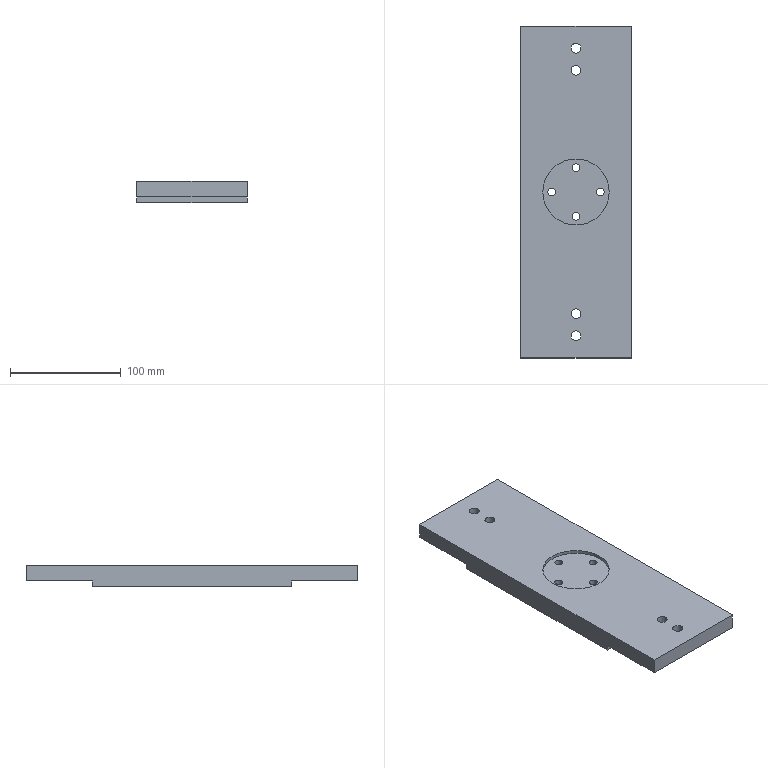Part | STEP file | SN10_010_002_SUPORTE | 1 solid | 20 faces | box 100 x 300 x 19 mm | volume 495492 mm3 | plane 11 | cylinder 9 | commonest cylinder face diameters 7 x4 9 x4 60 x1
STEP:
#1=CARTESIAN_POINT('',(0.,0.,0.));
#2=DIRECTION('',(0.,0.,1.));
#3=DIRECTION('',(1.,0.,0.));
#4=AXIS2_PLACEMENT_3D('',#1,#2,#3);
#5=CARTESIAN_POINT('',(25.072,1.678,300.));
#6=VERTEX_POINT('',#5);
#7=CARTESIAN_POINT('',(22.,0.,300.));
#8=DIRECTION('',(0.,0.,1.));
#9=DIRECTION('',(1.,0.,0.));
#10=AXIS2_PLACEMENT_3D('',#7,#8,#9);
#11=CIRCLE('',#10,3.5);
#12=CARTESIAN_POINT('',(22.,0.,300.1));
#13=DIRECTION('',(0.,0.,1.));
#14=DIRECTION('',(0.8776,0.4794,0.));
#15=AXIS2_PLACEMENT_3D('',#12,#13,#14);
#16=CYLINDRICAL_SURFACE('',#15,3.5);
#17=CARTESIAN_POINT('',(-0.5,-0.1));
#18=DIRECTION('',(1.,0.));
#19=VECTOR('',#18,1.);
#20=LINE('',#17,#19);
#21=(GEOMETRIC_REPRESENTATION_CONTEXT(2)PARAMETRIC_REPRESENTATION_CONTEXT()REPRESENTATION_CONTEXT('',''));
#22=DEFINITIONAL_REPRESENTATION('',(#20),#21);
#23=PCURVE('',#16,#22);
#24=CARTESIAN_POINT('',(0.,0.,300.));
#25=DIRECTION('',(0.,0.,1.));
#26=DIRECTION('',(1.,0.,0.));
#27=AXIS2_PLACEMENT_3D('',#24,#25,#26);
#28=PLANE('',#27);
#29=CARTESIAN_POINT('',(22.,0.));
#30=DIRECTION('',(1.,0.));
#31=AXIS2_PLACEMENT_2D('',#29,#30);
#32=CIRCLE('',#31,3.5);
#33=(GEOMETRIC_REPRESENTATION_CONTEXT(2)PARAMETRIC_REPRESENTATION_CONTEXT()REPRESENTATION_CONTEXT('',''));
#34=DEFINITIONAL_REPRESENTATION('',(#32),#33);
#35=PCURVE('',#28,#34);
#36=SURFACE_CURVE('',#11,(#23,#35),.PCURVE_S1.);
#37=EDGE_CURVE('',#6,#6,#36,.T.);
#38=ORIENTED_EDGE('',*,*,#37,.T.);
#39=CARTESIAN_POINT('',(25.072,1.678,316.));
#40=VERTEX_POINT('',#39);
#41=CARTESIAN_POINT('',(25.072,1.678,300.));
#42=CARTESIAN_POINT('',(25.072,1.678,316.));
#43=B_SPLINE_CURVE_WITH_KNOTS('',1,(#41,#42),.UNSPECIFIED.,.F.,.F.,(2,2),(-0.1,15.9),.PIECEWISE_BEZIER_KNOTS.);
#44=CARTESIAN_POINT('',(6.283,0.));
#45=DIRECTION('',(0.,1.));
#46=VECTOR('',#45,1.);
#47=LINE('',#44,#46);
#48=(GEOMETRIC_REPRESENTATION_CONTEXT(2)PARAMETRIC_REPRESENTATION_CONTEXT()REPRESENTATION_CONTEXT('',''));
#49=DEFINITIONAL_REPRESENTATION('',(#47),#48);
#50=PCURVE('',#16,#49);
#51=CARTESIAN_POINT('',(0.,0.));
#52=DIRECTION('',(0.,1.));
#53=VECTOR('',#52,1.);
#54=LINE('',#51,#53);
#55=(GEOMETRIC_REPRESENTATION_CONTEXT(2)PARAMETRIC_REPRESENTATION_CONTEXT()REPRESENTATION_CONTEXT('',''));
#56=DEFINITIONAL_REPRESENTATION('',(#54),#55);
#57=PCURVE('',#16,#56);
#58=SEAM_CURVE('',#43,(#50,#57),.PCURVE_S1.);
#59=EDGE_CURVE('',#6,#40,#58,.T.);
#60=ORIENTED_EDGE('',*,*,#59,.T.);
#61=CARTESIAN_POINT('',(22.,0.,316.));
#62=DIRECTION('',(0.,0.,1.));
#63=DIRECTION('',(1.,0.,0.));
#64=AXIS2_PLACEMENT_3D('',#61,#62,#63);
#65=CIRCLE('',#64,3.5);
#66=CARTESIAN_POINT('',(-0.5,15.9));
#67=DIRECTION('',(1.,0.));
#68=VECTOR('',#67,1.);
#69=LINE('',#66,#68);
#70=(GEOMETRIC_REPRESENTATION_CONTEXT(2)PARAMETRIC_REPRESENTATION_CONTEXT()REPRESENTATION_CONTEXT('',''));
#71=DEFINITIONAL_REPRESENTATION('',(#69),#70);
#72=PCURVE('',#16,#71);
#73=CARTESIAN_POINT('',(0.,0.,316.));
#74=DIRECTION('',(0.,0.,1.));
#75=DIRECTION('',(1.,0.,0.));
#76=AXIS2_PLACEMENT_3D('',#73,#74,#75);
#77=PLANE('',#76);
#78=CARTESIAN_POINT('',(22.,0.));
#79=DIRECTION('',(1.,0.));
#80=AXIS2_PLACEMENT_2D('',#78,#79);
#81=CIRCLE('',#80,3.5);
#82=(GEOMETRIC_REPRESENTATION_CONTEXT(2)PARAMETRIC_REPRESENTATION_CONTEXT()REPRESENTATION_CONTEXT('',''));
#83=DEFINITIONAL_REPRESENTATION('',(#81),#82);
#84=PCURVE('',#77,#83);
#85=SURFACE_CURVE('',#65,(#72,#84),.PCURVE_S1.);
#86=EDGE_CURVE('',#40,#40,#85,.T.);
#87=ORIENTED_EDGE('',*,*,#86,.F.);
#88=ORIENTED_EDGE('',*,*,#59,.F.);
#89=EDGE_LOOP('',(#38,#60,#87,#88));
#90=FACE_BOUND('',#89,.F.);
#91=ADVANCED_FACE('',(#90),#16,.F.);
#92=CARTESIAN_POINT('',(-30.,0.,316.));
#93=VERTEX_POINT('',#92);
#94=CARTESIAN_POINT('',(0.,0.,316.));
#95=DIRECTION('',(0.,0.,1.));
#96=DIRECTION('',(1.,0.,0.));
#97=AXIS2_PLACEMENT_3D('',#94,#95,#96);
#98=CIRCLE('',#97,30.);
#99=CARTESIAN_POINT('',(0.,0.,317.5));
#100=DIRECTION('',(0.,0.,1.));
#101=DIRECTION('',(1.,0.,0.));
#102=AXIS2_PLACEMENT_3D('',#99,#100,#101);
#103=CYLINDRICAL_SURFACE('',#102,30.);
#104=CARTESIAN_POINT('',(0.,-1.5));
#105=DIRECTION('',(1.,0.));
#106=VECTOR('',#105,1.);
#107=LINE('',#104,#106);
#108=(GEOMETRIC_REPRESENTATION_CONTEXT(2)PARAMETRIC_REPRESENTATION_CONTEXT()REPRESENTATION_CONTEXT('',''));
#109=DEFINITIONAL_REPRESENTATION('',(#107),#108);
#110=PCURVE('',#103,#109);
#111=CARTESIAN_POINT('',(0.,0.));
#112=DIRECTION('',(1.,0.));
#113=AXIS2_PLACEMENT_2D('',#111,#112);
#114=CIRCLE('',#113,30.);
#115=(GEOMETRIC_REPRESENTATION_CONTEXT(2)PARAMETRIC_REPRESENTATION_CONTEXT()REPRESENTATION_CONTEXT('',''));
#116=DEFINITIONAL_REPRESENTATION('',(#114),#115);
#117=PCURVE('',#77,#116);
#118=SURFACE_CURVE('',#98,(#110,#117),.PCURVE_S1.);
#119=EDGE_CURVE('',#93,#93,#118,.T.);
#120=ORIENTED_EDGE('',*,*,#119,.T.);
#121=CARTESIAN_POINT('',(-30.,0.,319.));
#122=VERTEX_POINT('',#121);
#123=CARTESIAN_POINT('',(-30.,0.,316.));
#124=CARTESIAN_POINT('',(-30.,0.,319.));
#125=B_SPLINE_CURVE_WITH_KNOTS('',1,(#123,#124),.UNSPECIFIED.,.F.,.F.,(2,2),(-1.5,1.5),.PIECEWISE_BEZIER_KNOTS.);
#126=CARTESIAN_POINT('',(9.425,0.));
#127=DIRECTION('',(0.,1.));
#128=VECTOR('',#127,1.);
#129=LINE('',#126,#128);
#130=(GEOMETRIC_REPRESENTATION_CONTEXT(2)PARAMETRIC_REPRESENTATION_CONTEXT()REPRESENTATION_CONTEXT('',''));
#131=DEFINITIONAL_REPRESENTATION('',(#129),#130);
#132=PCURVE('',#103,#131);
#133=CARTESIAN_POINT('',(3.142,0.));
#134=DIRECTION('',(0.,1.));
#135=VECTOR('',#134,1.);
#136=LINE('',#133,#135);
#137=(GEOMETRIC_REPRESENTATION_CONTEXT(2)PARAMETRIC_REPRESENTATION_CONTEXT()REPRESENTATION_CONTEXT('',''));
#138=DEFINITIONAL_REPRESENTATION('',(#136),#137);
#139=PCURVE('',#103,#138);
#140=SEAM_CURVE('',#125,(#132,#139),.PCURVE_S1.);
#141=EDGE_CURVE('',#93,#122,#140,.T.);
#142=ORIENTED_EDGE('',*,*,#141,.T.);
#143=CARTESIAN_POINT('',(0.,0.,319.));
#144=DIRECTION('',(0.,0.,1.));
#145=DIRECTION('',(1.,0.,0.));
#146=AXIS2_PLACEMENT_3D('',#143,#144,#145);
#147=CIRCLE('',#146,30.);
#148=CARTESIAN_POINT('',(0.,1.5));
#149=DIRECTION('',(1.,0.));
#150=VECTOR('',#149,1.);
#151=LINE('',#148,#150);
#152=(GEOMETRIC_REPRESENTATION_CONTEXT(2)PARAMETRIC_REPRESENTATION_CONTEXT()REPRESENTATION_CONTEXT('',''));
#153=DEFINITIONAL_REPRESENTATION('',(#151),#152);
#154=PCURVE('',#103,#153);
#155=CARTESIAN_POINT('',(0.,0.,319.));
#156=DIRECTION('',(0.,0.,1.));
#157=DIRECTION('',(1.,0.,0.));
#158=AXIS2_PLACEMENT_3D('',#155,#156,#157);
#159=PLANE('',#158);
#160=CARTESIAN_POINT('',(0.,0.));
#161=DIRECTION('',(1.,0.));
#162=AXIS2_PLACEMENT_2D('',#160,#161);
#163=CIRCLE('',#162,30.);
#164=(GEOMETRIC_REPRESENTATION_CONTEXT(2)PARAMETRIC_REPRESENTATION_CONTEXT()REPRESENTATION_CONTEXT('',''));
#165=DEFINITIONAL_REPRESENTATION('',(#163),#164);
#166=PCURVE('',#159,#165);
#167=SURFACE_CURVE('',#147,(#154,#166),.PCURVE_S1.);
#168=EDGE_CURVE('',#122,#122,#167,.T.);
#169=ORIENTED_EDGE('',*,*,#168,.F.);
#170=ORIENTED_EDGE('',*,*,#141,.F.);
#171=EDGE_LOOP('',(#120,#142,#169,#170));
#172=FACE_BOUND('',#171,.F.);
#173=ADVANCED_FACE('',(#172),#103,.F.);
#174=CARTESIAN_POINT('',(-50.,150.,319.));
#175=VERTEX_POINT('',#174);
#176=CARTESIAN_POINT('',(50.,150.,319.));
#177=VERTEX_POINT('',#176);
#178=CARTESIAN_POINT('',(-50.,150.,319.));
#179=DIRECTION('',(1.,0.,0.));
#180=VECTOR('',#179,1.);
#181=LINE('',#178,#180);
#182=CARTESIAN_POINT('',(-50.,150.));
#183=DIRECTION('',(1.,0.));
#184=VECTOR('',#183,1.);
#185=LINE('',#182,#184);
#186=(GEOMETRIC_REPRESENTATION_CONTEXT(2)PARAMETRIC_REPRESENTATION_CONTEXT()REPRESENTATION_CONTEXT('',''));
#187=DEFINITIONAL_REPRESENTATION('',(#185),#186);
#188=PCURVE('',#159,#187);
#189=CARTESIAN_POINT('',(-50.,150.,300.));
#190=DIRECTION('',(0.,-1.,0.));
#191=DIRECTION('',(0.,0.,-1.));
#192=AXIS2_PLACEMENT_3D('',#189,#190,#191);
#193=PLANE('',#192);
#194=CARTESIAN_POINT('',(-19.,0.));
#195=DIRECTION('',(0.,1.));
#196=VECTOR('',#195,1.);
#197=LINE('',#194,#196);
#198=(GEOMETRIC_REPRESENTATION_CONTEXT(2)PARAMETRIC_REPRESENTATION_CONTEXT()REPRESENTATION_CONTEXT('',''));
#199=DEFINITIONAL_REPRESENTATION('',(#197),#198);
#200=PCURVE('',#193,#199);
#201=SURFACE_CURVE('',#181,(#188,#200),.PCURVE_S1.);
#202=EDGE_CURVE('',#175,#177,#201,.T.);
#203=ORIENTED_EDGE('',*,*,#202,.F.);
#204=CARTESIAN_POINT('',(-50.,-150.,319.));
#205=VERTEX_POINT('',#204);
#206=CARTESIAN_POINT('',(-50.,150.,319.));
#207=DIRECTION('',(0.,-1.,0.));
#208=VECTOR('',#207,1.);
#209=LINE('',#206,#208);
#210=CARTESIAN_POINT('',(-50.,150.));
#211=DIRECTION('',(0.,-1.));
#212=VECTOR('',#211,1.);
#213=LINE('',#210,#212);
#214=(GEOMETRIC_REPRESENTATION_CONTEXT(2)PARAMETRIC_REPRESENTATION_CONTEXT()REPRESENTATION_CONTEXT('',''));
#215=DEFINITIONAL_REPRESENTATION('',(#213),#214);
#216=PCURVE('',#159,#215);
#217=CARTESIAN_POINT('',(-50.,150.,300.));
#218=DIRECTION('',(-1.,0.,0.));
#219=DIRECTION('',(0.,0.,1.));
#220=AXIS2_PLACEMENT_3D('',#217,#218,#219);
#221=PLANE('',#220);
#222=CARTESIAN_POINT('',(19.,0.));
#223=DIRECTION('',(0.,-1.));
#224=VECTOR('',#223,1.);
#225=LINE('',#222,#224);
#226=(GEOMETRIC_REPRESENTATION_CONTEXT(2)PARAMETRIC_REPRESENTATION_CONTEXT()REPRESENTATION_CONTEXT('',''));
#227=DEFINITIONAL_REPRESENTATION('',(#225),#226);
#228=PCURVE('',#221,#227);
#229=SURFACE_CURVE('',#209,(#216,#228),.PCURVE_S1.);
#230=EDGE_CURVE('',#175,#205,#229,.T.);
#231=ORIENTED_EDGE('',*,*,#230,.T.);
#232=CARTESIAN_POINT('',(50.,-150.,319.));
#233=VERTEX_POINT('',#232);
#234=CARTESIAN_POINT('',(-50.,-150.,319.));
#235=DIRECTION('',(1.,0.,0.));
#236=VECTOR('',#235,1.);
#237=LINE('',#234,#236);
#238=CARTESIAN_POINT('',(-50.,-150.));
#239=DIRECTION('',(1.,0.));
#240=VECTOR('',#239,1.);
#241=LINE('',#238,#240);
#242=(GEOMETRIC_REPRESENTATION_CONTEXT(2)PARAMETRIC_REPRESENTATION_CONTEXT()REPRESENTATION_CONTEXT('',''));
#243=DEFINITIONAL_REPRESENTATION('',(#241),#242);
#244=PCURVE('',#159,#243);
#245=CARTESIAN_POINT('',(-50.,-150.,300.));
#246=DIRECTION('',(0.,-1.,0.));
#247=DIRECTION('',(0.,0.,-1.));
#248=AXIS2_PLACEMENT_3D('',#245,#246,#247);
#249=PLANE('',#248);
#250=CARTESIAN_POINT('',(-19.,0.));
#251=DIRECTION('',(0.,1.));
#252=VECTOR('',#251,1.);
#253=LINE('',#250,#252);
#254=(GEOMETRIC_REPRESENTATION_CONTEXT(2)PARAMETRIC_REPRESENTATION_CONTEXT()REPRESENTATION_CONTEXT('',''));
#255=DEFINITIONAL_REPRESENTATION('',(#253),#254);
#256=PCURVE('',#249,#255);
#257=SURFACE_CURVE('',#237,(#244,#256),.PCURVE_S1.);
#258=EDGE_CURVE('',#205,#233,#257,.T.);
#259=ORIENTED_EDGE('',*,*,#258,.T.);
#260=CARTESIAN_POINT('',(50.,150.,319.));
#261=DIRECTION('',(0.,-1.,0.));
#262=VECTOR('',#261,1.);
#263=LINE('',#260,#262);
#264=CARTESIAN_POINT('',(50.,150.));
#265=DIRECTION('',(0.,-1.));
#266=VECTOR('',#265,1.);
#267=LINE('',#264,#266);
#268=(GEOMETRIC_REPRESENTATION_CONTEXT(2)PARAMETRIC_REPRESENTATION_CONTEXT()REPRESENTATION_CONTEXT('',''));
#269=DEFINITIONAL_REPRESENTATION('',(#267),#268);
#270=PCURVE('',#159,#269);
#271=CARTESIAN_POINT('',(50.,150.,300.));
#272=DIRECTION('',(-1.,0.,0.));
#273=DIRECTION('',(0.,0.,1.));
#274=AXIS2_PLACEMENT_3D('',#271,#272,#273);
#275=PLANE('',#274);
#276=CARTESIAN_POINT('',(19.,0.));
#277=DIRECTION('',(0.,-1.));
#278=VECTOR('',#277,1.);
#279=LINE('',#276,#278);
#280=(GEOMETRIC_REPRESENTATION_CONTEXT(2)PARAMETRIC_REPRESENTATION_CONTEXT()REPRESENTATION_CONTEXT('',''));
#281=DEFINITIONAL_REPRESENTATION('',(#279),#280);
#282=PCURVE('',#275,#281);
#283=SURFACE_CURVE('',#263,(#270,#282),.PCURVE_S1.);
#284=EDGE_CURVE('',#177,#233,#283,.T.);
#285=ORIENTED_EDGE('',*,*,#284,.F.);
#286=EDGE_LOOP('',(#203,#231,#259,#285));
#287=FACE_BOUND('',#286,.T.);
#288=ORIENTED_EDGE('',*,*,#168,.F.);
#289=EDGE_LOOP('',(#288));
#290=FACE_BOUND('',#289,.T.);
#291=CARTESIAN_POINT('',(-3.949,-107.843,319.));
#292=VERTEX_POINT('',#291);
#293=CARTESIAN_POINT('',(0.,-110.,319.));
#294=DIRECTION('',(0.,0.,1.));
#295=DIRECTION('',(1.,0.,0.));
#296=AXIS2_PLACEMENT_3D('',#293,#294,#295);
#297=CIRCLE('',#296,4.5);
#298=CARTESIAN_POINT('',(0.,-110.));
#299=DIRECTION('',(1.,0.));
#300=AXIS2_PLACEMENT_2D('',#298,#299);
#301=CIRCLE('',#300,4.5);
#302=(GEOMETRIC_REPRESENTATION_CONTEXT(2)PARAMETRIC_REPRESENTATION_CONTEXT()REPRESENTATION_CONTEXT('',''));
#303=DEFINITIONAL_REPRESENTATION('',(#301),#302);
#304=PCURVE('',#159,#303);
#305=CARTESIAN_POINT('',(0.,-110.,318.9));
#306=DIRECTION('',(0.,0.,-1.));
#307=DIRECTION('',(0.8776,-0.4794,0.));
#308=AXIS2_PLACEMENT_3D('',#305,#306,#307);
#309=CYLINDRICAL_SURFACE('',#308,4.5);
#310=CARTESIAN_POINT('',(12.066,-0.1));
#311=DIRECTION('',(-1.,0.));
#312=VECTOR('',#311,1.);
#313=LINE('',#310,#312);
#314=(GEOMETRIC_REPRESENTATION_CONTEXT(2)PARAMETRIC_REPRESENTATION_CONTEXT()REPRESENTATION_CONTEXT('',''));
#315=DEFINITIONAL_REPRESENTATION('',(#313),#314);
#316=PCURVE('',#309,#315);
#317=SURFACE_CURVE('',#297,(#304,#316),.PCURVE_S1.);
#318=EDGE_CURVE('',#292,#292,#317,.T.);
#319=ORIENTED_EDGE('',*,*,#318,.F.);
#320=EDGE_LOOP('',(#319));
#321=FACE_BOUND('',#320,.T.);
#322=CARTESIAN_POINT('',(3.949,-132.157,319.));
#323=VERTEX_POINT('',#322);
#324=CARTESIAN_POINT('',(0.,-130.,319.));
#325=DIRECTION('',(0.,0.,1.));
#326=DIRECTION('',(1.,0.,0.));
#327=AXIS2_PLACEMENT_3D('',#324,#325,#326);
#328=CIRCLE('',#327,4.5);
#329=CARTESIAN_POINT('',(0.,-130.));
#330=DIRECTION('',(1.,0.));
#331=AXIS2_PLACEMENT_2D('',#329,#330);
#332=CIRCLE('',#331,4.5);
#333=(GEOMETRIC_REPRESENTATION_CONTEXT(2)PARAMETRIC_REPRESENTATION_CONTEXT()REPRESENTATION_CONTEXT('',''));
#334=DEFINITIONAL_REPRESENTATION('',(#332),#333);
#335=PCURVE('',#159,#334);
#336=CARTESIAN_POINT('',(0.,-130.,318.9));
#337=DIRECTION('',(0.,0.,-1.));
#338=DIRECTION('',(0.8776,-0.4794,0.));
#339=AXIS2_PLACEMENT_3D('',#336,#337,#338);
#340=CYLINDRICAL_SURFACE('',#339,4.5);
#341=CARTESIAN_POINT('',(12.066,-0.1));
#342=DIRECTION('',(-1.,0.));
#343=VECTOR('',#342,1.);
#344=LINE('',#341,#343);
#345=(GEOMETRIC_REPRESENTATION_CONTEXT(2)PARAMETRIC_REPRESENTATION_CONTEXT()REPRESENTATION_CONTEXT('',''));
#346=DEFINITIONAL_REPRESENTATION('',(#344),#345);
#347=PCURVE('',#340,#346);
#348=SURFACE_CURVE('',#328,(#335,#347),.PCURVE_S1.);
#349=EDGE_CURVE('',#323,#323,#348,.T.);
#350=ORIENTED_EDGE('',*,*,#349,.F.);
#351=EDGE_LOOP('',(#350));
#352=FACE_BOUND('',#351,.T.);
#353=CARTESIAN_POINT('',(-3.949,112.157,319.));
#354=VERTEX_POINT('',#353);
#355=CARTESIAN_POINT('',(0.,110.,319.));
#356=DIRECTION('',(0.,0.,1.));
#357=DIRECTION('',(1.,0.,0.));
#358=AXIS2_PLACEMENT_3D('',#355,#356,#357);
#359=CIRCLE('',#358,4.5);
#360=CARTESIAN_POINT('',(0.,110.));
#361=DIRECTION('',(1.,0.));
#362=AXIS2_PLACEMENT_2D('',#360,#361);
#363=CIRCLE('',#362,4.5);
#364=(GEOMETRIC_REPRESENTATION_CONTEXT(2)PARAMETRIC_REPRESENTATION_CONTEXT()REPRESENTATION_CONTEXT('',''));
#365=DEFINITIONAL_REPRESENTATION('',(#363),#364);
#366=PCURVE('',#159,#365);
#367=CARTESIAN_POINT('',(0.,110.,318.9));
#368=DIRECTION('',(0.,0.,-1.));
#369=DIRECTION('',(0.8776,-0.4794,0.));
#370=AXIS2_PLACEMENT_3D('',#367,#368,#369);
#371=CYLINDRICAL_SURFACE('',#370,4.5);
#372=CARTESIAN_POINT('',(12.066,-0.1));
#373=DIRECTION('',(-1.,0.));
#374=VECTOR('',#373,1.);
#375=LINE('',#372,#374);
#376=(GEOMETRIC_REPRESENTATION_CONTEXT(2)PARAMETRIC_REPRESENTATION_CONTEXT()REPRESENTATION_CONTEXT('',''));
#377=DEFINITIONAL_REPRESENTATION('',(#375),#376);
#378=PCURVE('',#371,#377);
#379=SURFACE_CURVE('',#359,(#366,#378),.PCURVE_S1.);
#380=EDGE_CURVE('',#354,#354,#379,.T.);
#381=ORIENTED_EDGE('',*,*,#380,.F.);
#382=EDGE_LOOP('',(#381));
#383=FACE_BOUND('',#382,.T.);
#384=CARTESIAN_POINT('',(3.949,127.843,319.));
#385=VERTEX_POINT('',#384);
#386=CARTESIAN_POINT('',(0.,130.,319.));
#387=DIRECTION('',(0.,0.,1.));
#388=DIRECTION('',(1.,0.,0.));
#389=AXIS2_PLACEMENT_3D('',#386,#387,#388);
#390=CIRCLE('',#389,4.5);
#391=CARTESIAN_POINT('',(0.,130.));
#392=DIRECTION('',(1.,0.));
#393=AXIS2_PLACEMENT_2D('',#391,#392);
#394=CIRCLE('',#393,4.5);
#395=(GEOMETRIC_REPRESENTATION_CONTEXT(2)PARAMETRIC_REPRESENTATION_CONTEXT()REPRESENTATION_CONTEXT('',''));
#396=DEFINITIONAL_REPRESENTATION('',(#394),#395);
#397=PCURVE('',#159,#396);
#398=CARTESIAN_POINT('',(0.,130.,318.9));
#399=DIRECTION('',(0.,0.,-1.));
#400=DIRECTION('',(0.8776,-0.4794,0.));
#401=AXIS2_PLACEMENT_3D('',#398,#399,#400);
#402=CYLINDRICAL_SURFACE('',#401,4.5);
#403=CARTESIAN_POINT('',(12.066,-0.1));
#404=DIRECTION('',(-1.,0.));
#405=VECTOR('',#404,1.);
#406=LINE('',#403,#405);
#407=(GEOMETRIC_REPRESENTATION_CONTEXT(2)PARAMETRIC_REPRESENTATION_CONTEXT()REPRESENTATION_CONTEXT('',''));
#408=DEFINITIONAL_REPRESENTATION('',(#406),#407);
#409=PCURVE('',#402,#408);
#410=SURFACE_CURVE('',#390,(#397,#409),.PCURVE_S1.);
#411=EDGE_CURVE('',#385,#385,#410,.T.);
#412=ORIENTED_EDGE('',*,*,#411,.F.);
#413=EDGE_LOOP('',(#412));
#414=FACE_BOUND('',#413,.T.);
#415=ADVANCED_FACE('',(#287,#290,#321,#352,#383,#414),#159,.T.);
#416=ORIENTED_EDGE('',*,*,#119,.T.);
#417=EDGE_LOOP('',(#416));
#418=FACE_BOUND('',#417,.T.);
#419=ORIENTED_EDGE('',*,*,#86,.F.);
#420=EDGE_LOOP('',(#419));
#421=FACE_BOUND('',#420,.T.);
#422=CARTESIAN_POINT('',(-1.678,25.072,316.));
#423=VERTEX_POINT('',#422);
#424=CARTESIAN_POINT('',(0.,22.,316.));
#425=DIRECTION('',(0.,0.,1.));
#426=DIRECTION('',(1.,0.,0.));
#427=AXIS2_PLACEMENT_3D('',#424,#425,#426);
#428=CIRCLE('',#427,3.5);
#429=CARTESIAN_POINT('',(0.,22.));
#430=DIRECTION('',(1.,0.));
#431=AXIS2_PLACEMENT_2D('',#429,#430);
#432=CIRCLE('',#431,3.5);
#433=(GEOMETRIC_REPRESENTATION_CONTEXT(2)PARAMETRIC_REPRESENTATION_CONTEXT()REPRESENTATION_CONTEXT('',''));
#434=DEFINITIONAL_REPRESENTATION('',(#432),#433);
#435=PCURVE('',#77,#434);
#436=CARTESIAN_POINT('',(0.,22.,300.1));
#437=DIRECTION('',(0.,0.,1.));
#438=DIRECTION('',(-0.4794,0.8776,0.));
#439=AXIS2_PLACEMENT_3D('',#436,#437,#438);
#440=CYLINDRICAL_SURFACE('',#439,3.5);
#441=CARTESIAN_POINT('',(-2.071,15.9));
#442=DIRECTION('',(1.,0.));
#443=VECTOR('',#442,1.);
#444=LINE('',#441,#443);
#445=(GEOMETRIC_REPRESENTATION_CONTEXT(2)PARAMETRIC_REPRESENTATION_CONTEXT()REPRESENTATION_CONTEXT('',''));
#446=DEFINITIONAL_REPRESENTATION('',(#444),#445);
#447=PCURVE('',#440,#446);
#448=SURFACE_CURVE('',#428,(#435,#447),.PCURVE_S1.);
#449=EDGE_CURVE('',#423,#423,#448,.T.);
#450=ORIENTED_EDGE('',*,*,#449,.F.);
#451=EDGE_LOOP('',(#450));
#452=FACE_BOUND('',#451,.T.);
#453=CARTESIAN_POINT('',(-25.072,-1.678,316.));
#454=VERTEX_POINT('',#453);
#455=CARTESIAN_POINT('',(-22.,0.,316.));
#456=DIRECTION('',(0.,0.,1.));
#457=DIRECTION('',(1.,0.,0.));
#458=AXIS2_PLACEMENT_3D('',#455,#456,#457);
#459=CIRCLE('',#458,3.5);
#460=CARTESIAN_POINT('',(-22.,0.));
#461=DIRECTION('',(1.,0.));
#462=AXIS2_PLACEMENT_2D('',#460,#461);
#463=CIRCLE('',#462,3.5);
#464=(GEOMETRIC_REPRESENTATION_CONTEXT(2)PARAMETRIC_REPRESENTATION_CONTEXT()REPRESENTATION_CONTEXT('',''));
#465=DEFINITIONAL_REPRESENTATION('',(#463),#464);
#466=PCURVE('',#77,#465);
#467=CARTESIAN_POINT('',(-22.,0.,300.1));
#468=DIRECTION('',(0.,0.,1.));
#469=DIRECTION('',(-0.8776,-0.4794,0.));
#470=AXIS2_PLACEMENT_3D('',#467,#468,#469);
#471=CYLINDRICAL_SURFACE('',#470,3.5);
#472=CARTESIAN_POINT('',(-3.642,15.9));
#473=DIRECTION('',(1.,0.));
#474=VECTOR('',#473,1.);
#475=LINE('',#472,#474);
#476=(GEOMETRIC_REPRESENTATION_CONTEXT(2)PARAMETRIC_REPRESENTATION_CONTEXT()REPRESENTATION_CONTEXT('',''));
#477=DEFINITIONAL_REPRESENTATION('',(#475),#476);
#478=PCURVE('',#471,#477);
#479=SURFACE_CURVE('',#459,(#466,#478),.PCURVE_S1.);
#480=EDGE_CURVE('',#454,#454,#479,.T.);
#481=ORIENTED_EDGE('',*,*,#480,.F.);
#482=EDGE_LOOP('',(#481));
#483=FACE_BOUND('',#482,.T.);
#484=CARTESIAN_POINT('',(1.678,-25.072,316.));
#485=VERTEX_POINT('',#484);
#486=CARTESIAN_POINT('',(0.,-22.,316.));
#487=DIRECTION('',(0.,0.,1.));
#488=DIRECTION('',(1.,0.,0.));
#489=AXIS2_PLACEMENT_3D('',#486,#487,#488);
#490=CIRCLE('',#489,3.5);
#491=CARTESIAN_POINT('',(0.,-22.));
#492=DIRECTION('',(1.,0.));
#493=AXIS2_PLACEMENT_2D('',#491,#492);
#494=CIRCLE('',#493,3.5);
#495=(GEOMETRIC_REPRESENTATION_CONTEXT(2)PARAMETRIC_REPRESENTATION_CONTEXT()REPRESENTATION_CONTEXT('',''));
#496=DEFINITIONAL_REPRESENTATION('',(#494),#495);
#497=PCURVE('',#77,#496);
#498=CARTESIAN_POINT('',(0.,-22.,300.1));
#499=DIRECTION('',(0.,0.,1.));
#500=DIRECTION('',(0.4794,-0.8776,0.));
#501=AXIS2_PLACEMENT_3D('',#498,#499,#500);
#502=CYLINDRICAL_SURFACE('',#501,3.5);
#503=CARTESIAN_POINT('',(-5.212,15.9));
#504=DIRECTION('',(1.,0.));
#505=VECTOR('',#504,1.);
#506=LINE('',#503,#505);
#507=(GEOMETRIC_REPRESENTATION_CONTEXT(2)PARAMETRIC_REPRESENTATION_CONTEXT()REPRESENTATION_CONTEXT('',''));
#508=DEFINITIONAL_REPRESENTATION('',(#506),#507);
#509=PCURVE('',#502,#508);
#510=SURFACE_CURVE('',#490,(#497,#509),.PCURVE_S1.);
#511=EDGE_CURVE('',#485,#485,#510,.T.);
#512=ORIENTED_EDGE('',*,*,#511,.F.);
#513=EDGE_LOOP('',(#512));
#514=FACE_BOUND('',#513,.T.);
#515=ADVANCED_FACE('',(#418,#421,#452,#483,#514),#77,.T.);
#516=CARTESIAN_POINT('',(1.678,-25.072,300.));
#517=VERTEX_POINT('',#516);
#518=CARTESIAN_POINT('',(0.,-22.,300.));
#519=DIRECTION('',(0.,0.,1.));
#520=DIRECTION('',(1.,0.,0.));
#521=AXIS2_PLACEMENT_3D('',#518,#519,#520);
#522=CIRCLE('',#521,3.5);
#523=CARTESIAN_POINT('',(-5.212,-0.1));
#524=DIRECTION('',(1.,0.));
#525=VECTOR('',#524,1.);
#526=LINE('',#523,#525);
#527=(GEOMETRIC_REPRESENTATION_CONTEXT(2)PARAMETRIC_REPRESENTATION_CONTEXT()REPRESENTATION_CONTEXT('',''));
#528=DEFINITIONAL_REPRESENTATION('',(#526),#527);
#529=PCURVE('',#502,#528);
#530=CARTESIAN_POINT('',(0.,-22.));
#531=DIRECTION('',(1.,0.));
#532=AXIS2_PLACEMENT_2D('',#530,#531);
#533=CIRCLE('',#532,3.5);
#534=(GEOMETRIC_REPRESENTATION_CONTEXT(2)PARAMETRIC_REPRESENTATION_CONTEXT()REPRESENTATION_CONTEXT('',''));
#535=DEFINITIONAL_REPRESENTATION('',(#533),#534);
#536=PCURVE('',#28,#535);
#537=SURFACE_CURVE('',#522,(#529,#536),.PCURVE_S1.);
#538=EDGE_CURVE('',#517,#517,#537,.T.);
#539=ORIENTED_EDGE('',*,*,#538,.T.);
#540=CARTESIAN_POINT('',(1.678,-25.072,300.));
#541=CARTESIAN_POINT('',(1.678,-25.072,316.));
#542=B_SPLINE_CURVE_WITH_KNOTS('',1,(#540,#541),.UNSPECIFIED.,.F.,.F.,(2,2),(-0.1,15.9),.PIECEWISE_BEZIER_KNOTS.);
#543=CARTESIAN_POINT('',(6.283,0.));
#544=DIRECTION('',(0.,1.));
#545=VECTOR('',#544,1.);
#546=LINE('',#543,#545);
#547=(GEOMETRIC_REPRESENTATION_CONTEXT(2)PARAMETRIC_REPRESENTATION_CONTEXT()REPRESENTATION_CONTEXT('',''));
#548=DEFINITIONAL_REPRESENTATION('',(#546),#547);
#549=PCURVE('',#502,#548);
#550=CARTESIAN_POINT('',(0.,0.));
#551=DIRECTION('',(0.,1.));
#552=VECTOR('',#551,1.);
#553=LINE('',#550,#552);
#554=(GEOMETRIC_REPRESENTATION_CONTEXT(2)PARAMETRIC_REPRESENTATION_CONTEXT()REPRESENTATION_CONTEXT('',''));
#555=DEFINITIONAL_REPRESENTATION('',(#553),#554);
#556=PCURVE('',#502,#555);
#557=SEAM_CURVE('',#542,(#549,#556),.PCURVE_S1.);
#558=EDGE_CURVE('',#517,#485,#557,.T.);
#559=ORIENTED_EDGE('',*,*,#558,.T.);
#560=ORIENTED_EDGE('',*,*,#511,.F.);
#561=ORIENTED_EDGE('',*,*,#558,.F.);
#562=EDGE_LOOP('',(#539,#559,#560,#561));
#563=FACE_BOUND('',#562,.F.);
#564=ADVANCED_FACE('',(#563),#502,.F.);
#565=CARTESIAN_POINT('',(-25.072,-1.678,300.));
#566=VERTEX_POINT('',#565);
#567=CARTESIAN_POINT('',(-22.,0.,300.));
#568=DIRECTION('',(0.,0.,1.));
#569=DIRECTION('',(1.,0.,0.));
#570=AXIS2_PLACEMENT_3D('',#567,#568,#569);
#571=CIRCLE('',#570,3.5);
#572=CARTESIAN_POINT('',(-3.642,-0.1));
#573=DIRECTION('',(1.,0.));
#574=VECTOR('',#573,1.);
#575=LINE('',#572,#574);
#576=(GEOMETRIC_REPRESENTATION_CONTEXT(2)PARAMETRIC_REPRESENTATION_CONTEXT()REPRESENTATION_CONTEXT('',''));
#577=DEFINITIONAL_REPRESENTATION('',(#575),#576);
#578=PCURVE('',#471,#577);
#579=CARTESIAN_POINT('',(-22.,0.));
#580=DIRECTION('',(1.,0.));
#581=AXIS2_PLACEMENT_2D('',#579,#580);
#582=CIRCLE('',#581,3.5);
#583=(GEOMETRIC_REPRESENTATION_CONTEXT(2)PARAMETRIC_REPRESENTATION_CONTEXT()REPRESENTATION_CONTEXT('',''));
#584=DEFINITIONAL_REPRESENTATION('',(#582),#583);
#585=PCURVE('',#28,#584);
#586=SURFACE_CURVE('',#571,(#578,#585),.PCURVE_S1.);
#587=EDGE_CURVE('',#566,#566,#586,.T.);
#588=ORIENTED_EDGE('',*,*,#587,.T.);
#589=CARTESIAN_POINT('',(-25.072,-1.678,300.));
#590=CARTESIAN_POINT('',(-25.072,-1.678,316.));
#591=B_SPLINE_CURVE_WITH_KNOTS('',1,(#589,#590),.UNSPECIFIED.,.F.,.F.,(2,2),(-0.1,15.9),.PIECEWISE_BEZIER_KNOTS.);
#592=CARTESIAN_POINT('',(6.283,0.));
#593=DIRECTION('',(0.,1.));
#594=VECTOR('',#593,1.);
#595=LINE('',#592,#594);
#596=(GEOMETRIC_REPRESENTATION_CONTEXT(2)PARAMETRIC_REPRESENTATION_CONTEXT()REPRESENTATION_CONTEXT('',''));
#597=DEFINITIONAL_REPRESENTATION('',(#595),#596);
#598=PCURVE('',#471,#597);
#599=CARTESIAN_POINT('',(0.,0.));
#600=DIRECTION('',(0.,1.));
#601=VECTOR('',#600,1.);
#602=LINE('',#599,#601);
#603=(GEOMETRIC_REPRESENTATION_CONTEXT(2)PARAMETRIC_REPRESENTATION_CONTEXT()REPRESENTATION_CONTEXT('',''));
#604=DEFINITIONAL_REPRESENTATION('',(#602),#603);
#605=PCURVE('',#471,#604);
#606=SEAM_CURVE('',#591,(#598,#605),.PCURVE_S1.);
#607=EDGE_CURVE('',#566,#454,#606,.T.);
#608=ORIENTED_EDGE('',*,*,#607,.T.);
#609=ORIENTED_EDGE('',*,*,#480,.F.);
#610=ORIENTED_EDGE('',*,*,#607,.F.);
#611=EDGE_LOOP('',(#588,#608,#609,#610));
#612=FACE_BOUND('',#611,.F.);
#613=ADVANCED_FACE('',(#612),#471,.F.);
#614=CARTESIAN_POINT('',(-1.678,25.072,300.));
#615=VERTEX_POINT('',#614);
#616=CARTESIAN_POINT('',(0.,22.,300.));
#617=DIRECTION('',(0.,0.,1.));
#618=DIRECTION('',(1.,0.,0.));
#619=AXIS2_PLACEMENT_3D('',#616,#617,#618);
#620=CIRCLE('',#619,3.5);
#621=CARTESIAN_POINT('',(-2.071,-0.1));
#622=DIRECTION('',(1.,0.));
#623=VECTOR('',#622,1.);
#624=LINE('',#621,#623);
#625=(GEOMETRIC_REPRESENTATION_CONTEXT(2)PARAMETRIC_REPRESENTATION_CONTEXT()REPRESENTATION_CONTEXT('',''));
#626=DEFINITIONAL_REPRESENTATION('',(#624),#625);
#627=PCURVE('',#440,#626);
#628=CARTESIAN_POINT('',(0.,22.));
#629=DIRECTION('',(1.,0.));
#630=AXIS2_PLACEMENT_2D('',#628,#629);
#631=CIRCLE('',#630,3.5);
#632=(GEOMETRIC_REPRESENTATION_CONTEXT(2)PARAMETRIC_REPRESENTATION_CONTEXT()REPRESENTATION_CONTEXT('',''));
#633=DEFINITIONAL_REPRESENTATION('',(#631),#632);
#634=PCURVE('',#28,#633);
#635=SURFACE_CURVE('',#620,(#627,#634),.PCURVE_S1.);
#636=EDGE_CURVE('',#615,#615,#635,.T.);
#637=ORIENTED_EDGE('',*,*,#636,.T.);
#638=CARTESIAN_POINT('',(-1.678,25.072,300.));
#639=CARTESIAN_POINT('',(-1.678,25.072,316.));
#640=B_SPLINE_CURVE_WITH_KNOTS('',1,(#638,#639),.UNSPECIFIED.,.F.,.F.,(2,2),(-0.1,15.9),.PIECEWISE_BEZIER_KNOTS.);
#641=CARTESIAN_POINT('',(6.283,0.));
#642=DIRECTION('',(0.,1.));
#643=VECTOR('',#642,1.);
#644=LINE('',#641,#643);
#645=(GEOMETRIC_REPRESENTATION_CONTEXT(2)PARAMETRIC_REPRESENTATION_CONTEXT()REPRESENTATION_CONTEXT('',''));
#646=DEFINITIONAL_REPRESENTATION('',(#644),#645);
#647=PCURVE('',#440,#646);
#648=CARTESIAN_POINT('',(0.,0.));
#649=DIRECTION('',(0.,1.));
#650=VECTOR('',#649,1.);
#651=LINE('',#648,#650);
#652=(GEOMETRIC_REPRESENTATION_CONTEXT(2)PARAMETRIC_REPRESENTATION_CONTEXT()REPRESENTATION_CONTEXT('',''));
#653=DEFINITIONAL_REPRESENTATION('',(#651),#652);
#654=PCURVE('',#440,#653);
#655=SEAM_CURVE('',#640,(#647,#654),.PCURVE_S1.);
#656=EDGE_CURVE('',#615,#423,#655,.T.);
#657=ORIENTED_EDGE('',*,*,#656,.T.);
#658=ORIENTED_EDGE('',*,*,#449,.F.);
#659=ORIENTED_EDGE('',*,*,#656,.F.);
#660=EDGE_LOOP('',(#637,#657,#658,#659));
#661=FACE_BOUND('',#660,.F.);
#662=ADVANCED_FACE('',(#661),#440,.F.);
#663=CARTESIAN_POINT('',(-50.,90.,300.));
#664=VERTEX_POINT('',#663);
#665=CARTESIAN_POINT('',(-50.,-90.,300.));
#666=VERTEX_POINT('',#665);
#667=CARTESIAN_POINT('',(-50.,90.,300.));
#668=DIRECTION('',(0.,-1.,0.));
#669=VECTOR('',#668,1.);
#670=LINE('',#667,#669);
#671=CARTESIAN_POINT('',(-50.,90.));
#672=DIRECTION('',(0.,-1.));
#673=VECTOR('',#672,1.);
#674=LINE('',#671,#673);
#675=(GEOMETRIC_REPRESENTATION_CONTEXT(2)PARAMETRIC_REPRESENTATION_CONTEXT()REPRESENTATION_CONTEXT('',''));
#676=DEFINITIONAL_REPRESENTATION('',(#674),#675);
#677=PCURVE('',#28,#676);
#678=CARTESIAN_POINT('',(0.,-60.));
#679=DIRECTION('',(0.,-1.));
#680=VECTOR('',#679,1.);
#681=LINE('',#678,#680);
#682=(GEOMETRIC_REPRESENTATION_CONTEXT(2)PARAMETRIC_REPRESENTATION_CONTEXT()REPRESENTATION_CONTEXT('',''));
#683=DEFINITIONAL_REPRESENTATION('',(#681),#682);
#684=PCURVE('',#221,#683);
#685=SURFACE_CURVE('',#670,(#677,#684),.PCURVE_S1.);
#686=EDGE_CURVE('',#664,#666,#685,.T.);
#687=ORIENTED_EDGE('',*,*,#686,.F.);
#688=CARTESIAN_POINT('',(50.,90.,300.));
#689=VERTEX_POINT('',#688);
#690=CARTESIAN_POINT('',(-50.,90.,300.));
#691=DIRECTION('',(1.,0.,0.));
#692=VECTOR('',#691,1.);
#693=LINE('',#690,#692);
#694=CARTESIAN_POINT('',(-50.,90.));
#695=DIRECTION('',(1.,0.));
#696=VECTOR('',#695,1.);
#697=LINE('',#694,#696);
#698=(GEOMETRIC_REPRESENTATION_CONTEXT(2)PARAMETRIC_REPRESENTATION_CONTEXT()REPRESENTATION_CONTEXT('',''));
#699=DEFINITIONAL_REPRESENTATION('',(#697),#698);
#700=PCURVE('',#28,#699);
#701=CARTESIAN_POINT('',(-50.,90.,300.));
#702=DIRECTION('',(0.,-1.,0.));
#703=DIRECTION('',(0.,0.,-1.));
#704=AXIS2_PLACEMENT_3D('',#701,#702,#703);
#705=PLANE('',#704);
#706=CARTESIAN_POINT('',(0.,0.));
#707=DIRECTION('',(0.,1.));
#708=VECTOR('',#707,1.);
#709=LINE('',#706,#708);
#710=(GEOMETRIC_REPRESENTATION_CONTEXT(2)PARAMETRIC_REPRESENTATION_CONTEXT()REPRESENTATION_CONTEXT('',''));
#711=DEFINITIONAL_REPRESENTATION('',(#709),#710);
#712=PCURVE('',#705,#711);
#713=SURFACE_CURVE('',#693,(#700,#712),.PCURVE_S1.);
#714=EDGE_CURVE('',#664,#689,#713,.T.);
#715=ORIENTED_EDGE('',*,*,#714,.T.);
#716=CARTESIAN_POINT('',(50.,-90.,300.));
#717=VERTEX_POINT('',#716);
#718=CARTESIAN_POINT('',(50.,90.,300.));
#719=DIRECTION('',(0.,-1.,0.));
#720=VECTOR('',#719,1.);
#721=LINE('',#718,#720);
#722=CARTESIAN_POINT('',(50.,90.));
#723=DIRECTION('',(0.,-1.));
#724=VECTOR('',#723,1.);
#725=LINE('',#722,#724);
#726=(GEOMETRIC_REPRESENTATION_CONTEXT(2)PARAMETRIC_REPRESENTATION_CONTEXT()REPRESENTATION_CONTEXT('',''));
#727=DEFINITIONAL_REPRESENTATION('',(#725),#726);
#728=PCURVE('',#28,#727);
#729=CARTESIAN_POINT('',(0.,-60.));
#730=DIRECTION('',(0.,-1.));
#731=VECTOR('',#730,1.);
#732=LINE('',#729,#731);
#733=(GEOMETRIC_REPRESENTATION_CONTEXT(2)PARAMETRIC_REPRESENTATION_CONTEXT()REPRESENTATION_CONTEXT('',''));
#734=DEFINITIONAL_REPRESENTATION('',(#732),#733);
#735=PCURVE('',#275,#734);
#736=SURFACE_CURVE('',#721,(#728,#735),.PCURVE_S1.);
#737=EDGE_CURVE('',#689,#717,#736,.T.);
#738=ORIENTED_EDGE('',*,*,#737,.T.);
#739=CARTESIAN_POINT('',(50.,-90.,300.));
#740=DIRECTION('',(-1.,0.,0.));
#741=VECTOR('',#740,1.);
#742=LINE('',#739,#741);
#743=CARTESIAN_POINT('',(50.,-90.));
#744=DIRECTION('',(-1.,0.));
#745=VECTOR('',#744,1.);
#746=LINE('',#743,#745);
#747=(GEOMETRIC_REPRESENTATION_CONTEXT(2)PARAMETRIC_REPRESENTATION_CONTEXT()REPRESENTATION_CONTEXT('',''));
#748=DEFINITIONAL_REPRESENTATION('',(#746),#747);
#749=PCURVE('',#28,#748);
#750=CARTESIAN_POINT('',(50.,-90.,300.));
#751=DIRECTION('',(0.,1.,0.));
#752=DIRECTION('',(0.,0.,1.));
#753=AXIS2_PLACEMENT_3D('',#750,#751,#752);
#754=PLANE('',#753);
#755=CARTESIAN_POINT('',(0.,0.));
#756=DIRECTION('',(0.,-1.));
#757=VECTOR('',#756,1.);
#758=LINE('',#755,#757);
#759=(GEOMETRIC_REPRESENTATION_CONTEXT(2)PARAMETRIC_REPRESENTATION_CONTEXT()REPRESENTATION_CONTEXT('',''));
#760=DEFINITIONAL_REPRESENTATION('',(#758),#759);
#761=PCURVE('',#754,#760);
#762=SURFACE_CURVE('',#742,(#749,#761),.PCURVE_S1.);
#763=EDGE_CURVE('',#717,#666,#762,.T.);
#764=ORIENTED_EDGE('',*,*,#763,.T.);
#765=EDGE_LOOP('',(#687,#715,#738,#764));
#766=FACE_BOUND('',#765,.T.);
#767=ORIENTED_EDGE('',*,*,#37,.T.);
#768=EDGE_LOOP('',(#767));
#769=FACE_BOUND('',#768,.T.);
#770=ORIENTED_EDGE('',*,*,#636,.T.);
#771=EDGE_LOOP('',(#770));
#772=FACE_BOUND('',#771,.T.);
#773=ORIENTED_EDGE('',*,*,#587,.T.);
#774=EDGE_LOOP('',(#773));
#775=FACE_BOUND('',#774,.T.);
#776=ORIENTED_EDGE('',*,*,#538,.T.);
#777=EDGE_LOOP('',(#776));
#778=FACE_BOUND('',#777,.T.);
#779=ADVANCED_FACE('',(#766,#769,#772,#775,#778),#28,.F.);
#780=CARTESIAN_POINT('',(-3.949,-107.843,305.));
#781=VERTEX_POINT('',#780);
#782=CARTESIAN_POINT('',(0.,-110.,305.));
#783=DIRECTION('',(0.,0.,-1.));
#784=DIRECTION('',(1.,0.,0.));
#785=AXIS2_PLACEMENT_3D('',#782,#783,#784);
#786=CIRCLE('',#785,4.5);
#787=CARTESIAN_POINT('',(-0.5,13.9));
#788=DIRECTION('',(1.,0.));
#789=VECTOR('',#788,1.);
#790=LINE('',#787,#789);
#791=(GEOMETRIC_REPRESENTATION_CONTEXT(2)PARAMETRIC_REPRESENTATION_CONTEXT()REPRESENTATION_CONTEXT('',''));
#792=DEFINITIONAL_REPRESENTATION('',(#790),#791);
#793=PCURVE('',#309,#792);
#794=CARTESIAN_POINT('',(0.,0.,305.));
#795=DIRECTION('',(0.,0.,-1.));
#796=DIRECTION('',(-1.,0.,0.));
#797=AXIS2_PLACEMENT_3D('',#794,#795,#796);
#798=PLANE('',#797);
#799=CARTESIAN_POINT('',(0.,-110.));
#800=DIRECTION('',(-1.,0.));
#801=AXIS2_PLACEMENT_2D('',#799,#800);
#802=CIRCLE('',#801,4.5);
#803=(GEOMETRIC_REPRESENTATION_CONTEXT(2)PARAMETRIC_REPRESENTATION_CONTEXT()REPRESENTATION_CONTEXT('',''));
#804=DEFINITIONAL_REPRESENTATION('',(#802),#803);
#805=PCURVE('',#798,#804);
#806=SURFACE_CURVE('',#786,(#793,#805),.PCURVE_S1.);
#807=EDGE_CURVE('',#781,#781,#806,.T.);
#808=ORIENTED_EDGE('',*,*,#807,.F.);
#809=CARTESIAN_POINT('',(-3.949,-107.843,319.));
#810=CARTESIAN_POINT('',(-3.949,-107.843,305.));
#811=B_SPLINE_CURVE_WITH_KNOTS('',1,(#809,#810),.UNSPECIFIED.,.F.,.F.,(2,2),(-0.1,13.9),.PIECEWISE_BEZIER_KNOTS.);
#812=CARTESIAN_POINT('',(3.142,0.));
#813=DIRECTION('',(0.,1.));
#814=VECTOR('',#813,1.);
#815=LINE('',#812,#814);
#816=(GEOMETRIC_REPRESENTATION_CONTEXT(2)PARAMETRIC_REPRESENTATION_CONTEXT()REPRESENTATION_CONTEXT('',''));
#817=DEFINITIONAL_REPRESENTATION('',(#815),#816);
#818=PCURVE('',#309,#817);
#819=CARTESIAN_POINT('',(9.425,0.));
#820=DIRECTION('',(0.,1.));
#821=VECTOR('',#820,1.);
#822=LINE('',#819,#821);
#823=(GEOMETRIC_REPRESENTATION_CONTEXT(2)PARAMETRIC_REPRESENTATION_CONTEXT()REPRESENTATION_CONTEXT('',''));
#824=DEFINITIONAL_REPRESENTATION('',(#822),#823);
#825=PCURVE('',#309,#824);
#826=SEAM_CURVE('',#811,(#818,#825),.PCURVE_S1.);
#827=EDGE_CURVE('',#292,#781,#826,.T.);
#828=ORIENTED_EDGE('',*,*,#827,.F.);
#829=ORIENTED_EDGE('',*,*,#318,.F.);
#830=ORIENTED_EDGE('',*,*,#827,.T.);
#831=EDGE_LOOP('',(#808,#828,#829,#830));
#832=FACE_BOUND('',#831,.F.);
#833=ADVANCED_FACE('',(#832),#309,.F.);
#834=CARTESIAN_POINT('',(3.949,-132.157,305.));
#835=VERTEX_POINT('',#834);
#836=CARTESIAN_POINT('',(0.,-130.,305.));
#837=DIRECTION('',(0.,0.,-1.));
#838=DIRECTION('',(1.,0.,0.));
#839=AXIS2_PLACEMENT_3D('',#836,#837,#838);
#840=CIRCLE('',#839,4.5);
#841=CARTESIAN_POINT('',(-0.5,13.9));
#842=DIRECTION('',(1.,0.));
#843=VECTOR('',#842,1.);
#844=LINE('',#841,#843);
#845=(GEOMETRIC_REPRESENTATION_CONTEXT(2)PARAMETRIC_REPRESENTATION_CONTEXT()REPRESENTATION_CONTEXT('',''));
#846=DEFINITIONAL_REPRESENTATION('',(#844),#845);
#847=PCURVE('',#340,#846);
#848=CARTESIAN_POINT('',(0.,-130.));
#849=DIRECTION('',(-1.,0.));
#850=AXIS2_PLACEMENT_2D('',#848,#849);
#851=CIRCLE('',#850,4.5);
#852=(GEOMETRIC_REPRESENTATION_CONTEXT(2)PARAMETRIC_REPRESENTATION_CONTEXT()REPRESENTATION_CONTEXT('',''));
#853=DEFINITIONAL_REPRESENTATION('',(#851),#852);
#854=PCURVE('',#798,#853);
#855=SURFACE_CURVE('',#840,(#847,#854),.PCURVE_S1.);
#856=EDGE_CURVE('',#835,#835,#855,.T.);
#857=ORIENTED_EDGE('',*,*,#856,.F.);
#858=CARTESIAN_POINT('',(3.949,-132.157,319.));
#859=CARTESIAN_POINT('',(3.949,-132.157,305.));
#860=B_SPLINE_CURVE_WITH_KNOTS('',1,(#858,#859),.UNSPECIFIED.,.F.,.F.,(2,2),(-0.1,13.9),.PIECEWISE_BEZIER_KNOTS.);
#861=CARTESIAN_POINT('',(0.,0.));
#862=DIRECTION('',(0.,1.));
#863=VECTOR('',#862,1.);
#864=LINE('',#861,#863);
#865=(GEOMETRIC_REPRESENTATION_CONTEXT(2)PARAMETRIC_REPRESENTATION_CONTEXT()REPRESENTATION_CONTEXT('',''));
#866=DEFINITIONAL_REPRESENTATION('',(#864),#865);
#867=PCURVE('',#340,#866);
#868=CARTESIAN_POINT('',(6.283,0.));
#869=DIRECTION('',(0.,1.));
#870=VECTOR('',#869,1.);
#871=LINE('',#868,#870);
#872=(GEOMETRIC_REPRESENTATION_CONTEXT(2)PARAMETRIC_REPRESENTATION_CONTEXT()REPRESENTATION_CONTEXT('',''));
#873=DEFINITIONAL_REPRESENTATION('',(#871),#872);
#874=PCURVE('',#340,#873);
#875=SEAM_CURVE('',#860,(#867,#874),.PCURVE_S1.);
#876=EDGE_CURVE('',#323,#835,#875,.T.);
#877=ORIENTED_EDGE('',*,*,#876,.F.);
#878=ORIENTED_EDGE('',*,*,#349,.F.);
#879=ORIENTED_EDGE('',*,*,#876,.T.);
#880=EDGE_LOOP('',(#857,#877,#878,#879));
#881=FACE_BOUND('',#880,.F.);
#882=ADVANCED_FACE('',(#881),#340,.F.);
#883=CARTESIAN_POINT('',(-3.949,112.157,305.));
#884=VERTEX_POINT('',#883);
#885=CARTESIAN_POINT('',(0.,110.,305.));
#886=DIRECTION('',(0.,0.,-1.));
#887=DIRECTION('',(1.,0.,0.));
#888=AXIS2_PLACEMENT_3D('',#885,#886,#887);
#889=CIRCLE('',#888,4.5);
#890=CARTESIAN_POINT('',(-0.5,13.9));
#891=DIRECTION('',(1.,0.));
#892=VECTOR('',#891,1.);
#893=LINE('',#890,#892);
#894=(GEOMETRIC_REPRESENTATION_CONTEXT(2)PARAMETRIC_REPRESENTATION_CONTEXT()REPRESENTATION_CONTEXT('',''));
#895=DEFINITIONAL_REPRESENTATION('',(#893),#894);
#896=PCURVE('',#371,#895);
#897=CARTESIAN_POINT('',(0.,0.,305.));
#898=DIRECTION('',(0.,0.,-1.));
#899=DIRECTION('',(-1.,0.,0.));
#900=AXIS2_PLACEMENT_3D('',#897,#898,#899);
#901=PLANE('',#900);
#902=CARTESIAN_POINT('',(0.,110.));
#903=DIRECTION('',(-1.,0.));
#904=AXIS2_PLACEMENT_2D('',#902,#903);
#905=CIRCLE('',#904,4.5);
#906=(GEOMETRIC_REPRESENTATION_CONTEXT(2)PARAMETRIC_REPRESENTATION_CONTEXT()REPRESENTATION_CONTEXT('',''));
#907=DEFINITIONAL_REPRESENTATION('',(#905),#906);
#908=PCURVE('',#901,#907);
#909=SURFACE_CURVE('',#889,(#896,#908),.PCURVE_S1.);
#910=EDGE_CURVE('',#884,#884,#909,.T.);
#911=ORIENTED_EDGE('',*,*,#910,.F.);
#912=CARTESIAN_POINT('',(-3.949,112.157,319.));
#913=CARTESIAN_POINT('',(-3.949,112.157,305.));
#914=B_SPLINE_CURVE_WITH_KNOTS('',1,(#912,#913),.UNSPECIFIED.,.F.,.F.,(2,2),(-0.1,13.9),.PIECEWISE_BEZIER_KNOTS.);
#915=CARTESIAN_POINT('',(3.142,0.));
#916=DIRECTION('',(0.,1.));
#917=VECTOR('',#916,1.);
#918=LINE('',#915,#917);
#919=(GEOMETRIC_REPRESENTATION_CONTEXT(2)PARAMETRIC_REPRESENTATION_CONTEXT()REPRESENTATION_CONTEXT('',''));
#920=DEFINITIONAL_REPRESENTATION('',(#918),#919);
#921=PCURVE('',#371,#920);
#922=CARTESIAN_POINT('',(9.425,0.));
#923=DIRECTION('',(0.,1.));
#924=VECTOR('',#923,1.);
#925=LINE('',#922,#924);
#926=(GEOMETRIC_REPRESENTATION_CONTEXT(2)PARAMETRIC_REPRESENTATION_CONTEXT()REPRESENTATION_CONTEXT('',''));
#927=DEFINITIONAL_REPRESENTATION('',(#925),#926);
#928=PCURVE('',#371,#927);
#929=SEAM_CURVE('',#914,(#921,#928),.PCURVE_S1.);
#930=EDGE_CURVE('',#354,#884,#929,.T.);
#931=ORIENTED_EDGE('',*,*,#930,.F.);
#932=ORIENTED_EDGE('',*,*,#380,.F.);
#933=ORIENTED_EDGE('',*,*,#930,.T.);
#934=EDGE_LOOP('',(#911,#931,#932,#933));
#935=FACE_BOUND('',#934,.F.);
#936=ADVANCED_FACE('',(#935),#371,.F.);
#937=CARTESIAN_POINT('',(3.949,127.843,305.));
#938=VERTEX_POINT('',#937);
#939=CARTESIAN_POINT('',(0.,130.,305.));
#940=DIRECTION('',(0.,0.,-1.));
#941=DIRECTION('',(1.,0.,0.));
#942=AXIS2_PLACEMENT_3D('',#939,#940,#941);
#943=CIRCLE('',#942,4.5);
#944=CARTESIAN_POINT('',(-0.5,13.9));
#945=DIRECTION('',(1.,0.));
#946=VECTOR('',#945,1.);
#947=LINE('',#944,#946);
#948=(GEOMETRIC_REPRESENTATION_CONTEXT(2)PARAMETRIC_REPRESENTATION_CONTEXT()REPRESENTATION_CONTEXT('',''));
#949=DEFINITIONAL_REPRESENTATION('',(#947),#948);
#950=PCURVE('',#402,#949);
#951=CARTESIAN_POINT('',(0.,130.));
#952=DIRECTION('',(-1.,0.));
#953=AXIS2_PLACEMENT_2D('',#951,#952);
#954=CIRCLE('',#953,4.5);
#955=(GEOMETRIC_REPRESENTATION_CONTEXT(2)PARAMETRIC_REPRESENTATION_CONTEXT()REPRESENTATION_CONTEXT('',''));
#956=DEFINITIONAL_REPRESENTATION('',(#954),#955);
#957=PCURVE('',#901,#956);
#958=SURFACE_CURVE('',#943,(#950,#957),.PCURVE_S1.);
#959=EDGE_CURVE('',#938,#938,#958,.T.);
#960=ORIENTED_EDGE('',*,*,#959,.F.);
#961=CARTESIAN_POINT('',(3.949,127.843,319.));
#962=CARTESIAN_POINT('',(3.949,127.843,305.));
#963=B_SPLINE_CURVE_WITH_KNOTS('',1,(#961,#962),.UNSPECIFIED.,.F.,.F.,(2,2),(-0.1,13.9),.PIECEWISE_BEZIER_KNOTS.);
#964=CARTESIAN_POINT('',(0.,0.));
#965=DIRECTION('',(0.,1.));
#966=VECTOR('',#965,1.);
#967=LINE('',#964,#966);
#968=(GEOMETRIC_REPRESENTATION_CONTEXT(2)PARAMETRIC_REPRESENTATION_CONTEXT()REPRESENTATION_CONTEXT('',''));
#969=DEFINITIONAL_REPRESENTATION('',(#967),#968);
#970=PCURVE('',#402,#969);
#971=CARTESIAN_POINT('',(6.283,0.));
#972=DIRECTION('',(0.,1.));
#973=VECTOR('',#972,1.);
#974=LINE('',#971,#973);
#975=(GEOMETRIC_REPRESENTATION_CONTEXT(2)PARAMETRIC_REPRESENTATION_CONTEXT()REPRESENTATION_CONTEXT('',''));
#976=DEFINITIONAL_REPRESENTATION('',(#974),#975);
#977=PCURVE('',#402,#976);
#978=SEAM_CURVE('',#963,(#970,#977),.PCURVE_S1.);
#979=EDGE_CURVE('',#385,#938,#978,.T.);
#980=ORIENTED_EDGE('',*,*,#979,.F.);
#981=ORIENTED_EDGE('',*,*,#411,.F.);
#982=ORIENTED_EDGE('',*,*,#979,.T.);
#983=EDGE_LOOP('',(#960,#980,#981,#982));
#984=FACE_BOUND('',#983,.F.);
#985=ADVANCED_FACE('',(#984),#402,.F.);
#986=CARTESIAN_POINT('',(50.,90.,305.));
#987=VERTEX_POINT('',#986);
#988=CARTESIAN_POINT('',(50.,90.,300.));
#989=DIRECTION('',(0.,0.,1.));
#990=VECTOR('',#989,1.);
#991=LINE('',#988,#990);
#992=CARTESIAN_POINT('',(0.,-60.));
#993=DIRECTION('',(1.,0.));
#994=VECTOR('',#993,1.);
#995=LINE('',#992,#994);
#996=(GEOMETRIC_REPRESENTATION_CONTEXT(2)PARAMETRIC_REPRESENTATION_CONTEXT()REPRESENTATION_CONTEXT('',''));
#997=DEFINITIONAL_REPRESENTATION('',(#995),#996);
#998=PCURVE('',#275,#997);
#999=CARTESIAN_POINT('',(0.,100.));
#1000=DIRECTION('',(-1.,0.));
#1001=VECTOR('',#1000,1.);
#1002=LINE('',#999,#1001);
#1003=(GEOMETRIC_REPRESENTATION_CONTEXT(2)PARAMETRIC_REPRESENTATION_CONTEXT()REPRESENTATION_CONTEXT('',''));
#1004=DEFINITIONAL_REPRESENTATION('',(#1002),#1003);
#1005=PCURVE('',#705,#1004);
#1006=SURFACE_CURVE('',#991,(#998,#1005),.PCURVE_S1.);
#1007=EDGE_CURVE('',#689,#987,#1006,.T.);
#1008=ORIENTED_EDGE('',*,*,#1007,.T.);
#1009=CARTESIAN_POINT('',(50.,150.,305.));
#1010=VERTEX_POINT('',#1009);
#1011=CARTESIAN_POINT('',(50.,150.,305.));
#1012=DIRECTION('',(0.,-1.,0.));
#1013=VECTOR('',#1012,1.);
#1014=LINE('',#1011,#1013);
#1015=CARTESIAN_POINT('',(5.,0.));
#1016=DIRECTION('',(0.,-1.));
#1017=VECTOR('',#1016,1.);
#1018=LINE('',#1015,#1017);
#1019=(GEOMETRIC_REPRESENTATION_CONTEXT(2)PARAMETRIC_REPRESENTATION_CONTEXT()REPRESENTATION_CONTEXT('',''));
#1020=DEFINITIONAL_REPRESENTATION('',(#1018),#1019);
#1021=PCURVE('',#275,#1020);
#1022=CARTESIAN_POINT('',(-50.,150.));
#1023=DIRECTION('',(0.,-1.));
#1024=VECTOR('',#1023,1.);
#1025=LINE('',#1022,#1024);
#1026=(GEOMETRIC_REPRESENTATION_CONTEXT(2)PARAMETRIC_REPRESENTATION_CONTEXT()REPRESENTATION_CONTEXT('',''));
#1027=DEFINITIONAL_REPRESENTATION('',(#1025),#1026);
#1028=PCURVE('',#901,#1027);
#1029=SURFACE_CURVE('',#1014,(#1021,#1028),.PCURVE_S1.);
#1030=EDGE_CURVE('',#1010,#987,#1029,.T.);
#1031=ORIENTED_EDGE('',*,*,#1030,.F.);
#1032=CARTESIAN_POINT('',(50.,150.,305.));
#1033=DIRECTION('',(0.,0.,1.));
#1034=VECTOR('',#1033,1.);
#1035=LINE('',#1032,#1034);
#1036=CARTESIAN_POINT('',(5.,0.));
#1037=DIRECTION('',(1.,0.));
#1038=VECTOR('',#1037,1.);
#1039=LINE('',#1036,#1038);
#1040=(GEOMETRIC_REPRESENTATION_CONTEXT(2)PARAMETRIC_REPRESENTATION_CONTEXT()REPRESENTATION_CONTEXT('',''));
#1041=DEFINITIONAL_REPRESENTATION('',(#1039),#1040);
#1042=PCURVE('',#275,#1041);
#1043=CARTESIAN_POINT('',(-5.,100.));
#1044=DIRECTION('',(-1.,0.));
#1045=VECTOR('',#1044,1.);
#1046=LINE('',#1043,#1045);
#1047=(GEOMETRIC_REPRESENTATION_CONTEXT(2)PARAMETRIC_REPRESENTATION_CONTEXT()REPRESENTATION_CONTEXT('',''));
#1048=DEFINITIONAL_REPRESENTATION('',(#1046),#1047);
#1049=PCURVE('',#193,#1048);
#1050=SURFACE_CURVE('',#1035,(#1042,#1049),.PCURVE_S1.);
#1051=EDGE_CURVE('',#1010,#177,#1050,.T.);
#1052=ORIENTED_EDGE('',*,*,#1051,.T.);
#1053=ORIENTED_EDGE('',*,*,#284,.T.);
#1054=CARTESIAN_POINT('',(50.,-150.,305.));
#1055=VERTEX_POINT('',#1054);
#1056=CARTESIAN_POINT('',(50.,-150.,305.));
#1057=DIRECTION('',(0.,0.,1.));
#1058=VECTOR('',#1057,1.);
#1059=LINE('',#1056,#1058);
#1060=CARTESIAN_POINT('',(5.,-300.));
#1061=DIRECTION('',(1.,0.));
#1062=VECTOR('',#1061,1.);
#1063=LINE('',#1060,#1062);
#1064=(GEOMETRIC_REPRESENTATION_CONTEXT(2)PARAMETRIC_REPRESENTATION_CONTEXT()REPRESENTATION_CONTEXT('',''));
#1065=DEFINITIONAL_REPRESENTATION('',(#1063),#1064);
#1066=PCURVE('',#275,#1065);
#1067=CARTESIAN_POINT('',(-5.,100.));
#1068=DIRECTION('',(-1.,0.));
#1069=VECTOR('',#1068,1.);
#1070=LINE('',#1067,#1069);
#1071=(GEOMETRIC_REPRESENTATION_CONTEXT(2)PARAMETRIC_REPRESENTATION_CONTEXT()REPRESENTATION_CONTEXT('',''));
#1072=DEFINITIONAL_REPRESENTATION('',(#1070),#1071);
#1073=PCURVE('',#249,#1072);
#1074=SURFACE_CURVE('',#1059,(#1066,#1073),.PCURVE_S1.);
#1075=EDGE_CURVE('',#1055,#233,#1074,.T.);
#1076=ORIENTED_EDGE('',*,*,#1075,.F.);
#1077=CARTESIAN_POINT('',(50.,-90.,305.));
#1078=VERTEX_POINT('',#1077);
#1079=CARTESIAN_POINT('',(50.,-90.,305.));
#1080=DIRECTION('',(0.,-1.,0.));
#1081=VECTOR('',#1080,1.);
#1082=LINE('',#1079,#1081);
#1083=CARTESIAN_POINT('',(5.,-240.));
#1084=DIRECTION('',(0.,-1.));
#1085=VECTOR('',#1084,1.);
#1086=LINE('',#1083,#1085);
#1087=(GEOMETRIC_REPRESENTATION_CONTEXT(2)PARAMETRIC_REPRESENTATION_CONTEXT()REPRESENTATION_CONTEXT('',''));
#1088=DEFINITIONAL_REPRESENTATION('',(#1086),#1087);
#1089=PCURVE('',#275,#1088);
#1090=CARTESIAN_POINT('',(-50.,-90.));
#1091=DIRECTION('',(0.,-1.));
#1092=VECTOR('',#1091,1.);
#1093=LINE('',#1090,#1092);
#1094=(GEOMETRIC_REPRESENTATION_CONTEXT(2)PARAMETRIC_REPRESENTATION_CONTEXT()REPRESENTATION_CONTEXT('',''));
#1095=DEFINITIONAL_REPRESENTATION('',(#1093),#1094);
#1096=PCURVE('',#798,#1095);
#1097=SURFACE_CURVE('',#1082,(#1089,#1096),.PCURVE_S1.);
#1098=EDGE_CURVE('',#1078,#1055,#1097,.T.);
#1099=ORIENTED_EDGE('',*,*,#1098,.F.);
#1100=CARTESIAN_POINT('',(50.,-90.,300.));
#1101=DIRECTION('',(0.,0.,1.));
#1102=VECTOR('',#1101,1.);
#1103=LINE('',#1100,#1102);
#1104=CARTESIAN_POINT('',(0.,-240.));
#1105=DIRECTION('',(1.,0.));
#1106=VECTOR('',#1105,1.);
#1107=LINE('',#1104,#1106);
#1108=(GEOMETRIC_REPRESENTATION_CONTEXT(2)PARAMETRIC_REPRESENTATION_CONTEXT()REPRESENTATION_CONTEXT('',''));
#1109=DEFINITIONAL_REPRESENTATION('',(#1107),#1108);
#1110=PCURVE('',#275,#1109);
#1111=CARTESIAN_POINT('',(0.,0.));
#1112=DIRECTION('',(1.,0.));
#1113=VECTOR('',#1112,1.);
#1114=LINE('',#1111,#1113);
#1115=(GEOMETRIC_REPRESENTATION_CONTEXT(2)PARAMETRIC_REPRESENTATION_CONTEXT()REPRESENTATION_CONTEXT('',''));
#1116=DEFINITIONAL_REPRESENTATION('',(#1114),#1115);
#1117=PCURVE('',#754,#1116);
#1118=SURFACE_CURVE('',#1103,(#1110,#1117),.PCURVE_S1.);
#1119=EDGE_CURVE('',#717,#1078,#1118,.T.);
#1120=ORIENTED_EDGE('',*,*,#1119,.F.);
#1121=ORIENTED_EDGE('',*,*,#737,.F.);
#1122=EDGE_LOOP('',(#1008,#1031,#1052,#1053,#1076,#1099,#1120,#1121));
#1123=FACE_BOUND('',#1122,.T.);
#1124=ADVANCED_FACE('',(#1123),#275,.F.);
#1125=ORIENTED_EDGE('',*,*,#1075,.T.);
#1126=ORIENTED_EDGE('',*,*,#258,.F.);
#1127=CARTESIAN_POINT('',(-50.,-150.,305.));
#1128=VERTEX_POINT('',#1127);
#1129=CARTESIAN_POINT('',(-50.,-150.,305.));
#1130=DIRECTION('',(0.,0.,1.));
#1131=VECTOR('',#1130,1.);
#1132=LINE('',#1129,#1131);
#1133=CARTESIAN_POINT('',(-5.,0.));
#1134=DIRECTION('',(-1.,0.));
#1135=VECTOR('',#1134,1.);
#1136=LINE('',#1133,#1135);
#1137=(GEOMETRIC_REPRESENTATION_CONTEXT(2)PARAMETRIC_REPRESENTATION_CONTEXT()REPRESENTATION_CONTEXT('',''));
#1138=DEFINITIONAL_REPRESENTATION('',(#1136),#1137);
#1139=PCURVE('',#249,#1138);
#1140=CARTESIAN_POINT('',(5.,-300.));
#1141=DIRECTION('',(1.,0.));
#1142=VECTOR('',#1141,1.);
#1143=LINE('',#1140,#1142);
#1144=(GEOMETRIC_REPRESENTATION_CONTEXT(2)PARAMETRIC_REPRESENTATION_CONTEXT()REPRESENTATION_CONTEXT('',''));
#1145=DEFINITIONAL_REPRESENTATION('',(#1143),#1144);
#1146=PCURVE('',#221,#1145);
#1147=SURFACE_CURVE('',#1132,(#1139,#1146),.PCURVE_S1.);
#1148=EDGE_CURVE('',#1128,#205,#1147,.T.);
#1149=ORIENTED_EDGE('',*,*,#1148,.F.);
#1150=CARTESIAN_POINT('',(-50.,-150.,305.));
#1151=DIRECTION('',(1.,0.,0.));
#1152=VECTOR('',#1151,1.);
#1153=LINE('',#1150,#1152);
#1154=CARTESIAN_POINT('',(-5.,0.));
#1155=DIRECTION('',(0.,1.));
#1156=VECTOR('',#1155,1.);
#1157=LINE('',#1154,#1156);
#1158=(GEOMETRIC_REPRESENTATION_CONTEXT(2)PARAMETRIC_REPRESENTATION_CONTEXT()REPRESENTATION_CONTEXT('',''));
#1159=DEFINITIONAL_REPRESENTATION('',(#1157),#1158);
#1160=PCURVE('',#249,#1159);
#1161=CARTESIAN_POINT('',(50.,-150.));
#1162=DIRECTION('',(-1.,0.));
#1163=VECTOR('',#1162,1.);
#1164=LINE('',#1161,#1163);
#1165=(GEOMETRIC_REPRESENTATION_CONTEXT(2)PARAMETRIC_REPRESENTATION_CONTEXT()REPRESENTATION_CONTEXT('',''));
#1166=DEFINITIONAL_REPRESENTATION('',(#1164),#1165);
#1167=PCURVE('',#798,#1166);
#1168=SURFACE_CURVE('',#1153,(#1160,#1167),.PCURVE_S1.);
#1169=EDGE_CURVE('',#1128,#1055,#1168,.T.);
#1170=ORIENTED_EDGE('',*,*,#1169,.T.);
#1171=EDGE_LOOP('',(#1125,#1126,#1149,#1170));
#1172=FACE_BOUND('',#1171,.T.);
#1173=ADVANCED_FACE('',(#1172),#249,.T.);
#1174=ORIENTED_EDGE('',*,*,#686,.T.);
#1175=CARTESIAN_POINT('',(-50.,-90.,305.));
#1176=VERTEX_POINT('',#1175);
#1177=CARTESIAN_POINT('',(-50.,-90.,300.));
#1178=DIRECTION('',(0.,0.,1.));
#1179=VECTOR('',#1178,1.);
#1180=LINE('',#1177,#1179);
#1181=CARTESIAN_POINT('',(0.,-240.));
#1182=DIRECTION('',(1.,0.));
#1183=VECTOR('',#1182,1.);
#1184=LINE('',#1181,#1183);
#1185=(GEOMETRIC_REPRESENTATION_CONTEXT(2)PARAMETRIC_REPRESENTATION_CONTEXT()REPRESENTATION_CONTEXT('',''));
#1186=DEFINITIONAL_REPRESENTATION('',(#1184),#1185);
#1187=PCURVE('',#221,#1186);
#1188=CARTESIAN_POINT('',(0.,-100.));
#1189=DIRECTION('',(1.,0.));
#1190=VECTOR('',#1189,1.);
#1191=LINE('',#1188,#1190);
#1192=(GEOMETRIC_REPRESENTATION_CONTEXT(2)PARAMETRIC_REPRESENTATION_CONTEXT()REPRESENTATION_CONTEXT('',''));
#1193=DEFINITIONAL_REPRESENTATION('',(#1191),#1192);
#1194=PCURVE('',#754,#1193);
#1195=SURFACE_CURVE('',#1180,(#1187,#1194),.PCURVE_S1.);
#1196=EDGE_CURVE('',#666,#1176,#1195,.T.);
#1197=ORIENTED_EDGE('',*,*,#1196,.T.);
#1198=CARTESIAN_POINT('',(-50.,-150.,305.));
#1199=DIRECTION('',(0.,1.,0.));
#1200=VECTOR('',#1199,1.);
#1201=LINE('',#1198,#1200);
#1202=CARTESIAN_POINT('',(5.,-300.));
#1203=DIRECTION('',(0.,1.));
#1204=VECTOR('',#1203,1.);
#1205=LINE('',#1202,#1204);
#1206=(GEOMETRIC_REPRESENTATION_CONTEXT(2)PARAMETRIC_REPRESENTATION_CONTEXT()REPRESENTATION_CONTEXT('',''));
#1207=DEFINITIONAL_REPRESENTATION('',(#1205),#1206);
#1208=PCURVE('',#221,#1207);
#1209=CARTESIAN_POINT('',(50.,-150.));
#1210=DIRECTION('',(0.,1.));
#1211=VECTOR('',#1210,1.);
#1212=LINE('',#1209,#1211);
#1213=(GEOMETRIC_REPRESENTATION_CONTEXT(2)PARAMETRIC_REPRESENTATION_CONTEXT()REPRESENTATION_CONTEXT('',''));
#1214=DEFINITIONAL_REPRESENTATION('',(#1212),#1213);
#1215=PCURVE('',#798,#1214);
#1216=SURFACE_CURVE('',#1201,(#1208,#1215),.PCURVE_S1.);
#1217=EDGE_CURVE('',#1128,#1176,#1216,.T.);
#1218=ORIENTED_EDGE('',*,*,#1217,.F.);
#1219=ORIENTED_EDGE('',*,*,#1148,.T.);
#1220=ORIENTED_EDGE('',*,*,#230,.F.);
#1221=CARTESIAN_POINT('',(-50.,150.,305.));
#1222=VERTEX_POINT('',#1221);
#1223=CARTESIAN_POINT('',(-50.,150.,305.));
#1224=DIRECTION('',(0.,0.,1.));
#1225=VECTOR('',#1224,1.);
#1226=LINE('',#1223,#1225);
#1227=CARTESIAN_POINT('',(5.,0.));
#1228=DIRECTION('',(1.,0.));
#1229=VECTOR('',#1228,1.);
#1230=LINE('',#1227,#1229);
#1231=(GEOMETRIC_REPRESENTATION_CONTEXT(2)PARAMETRIC_REPRESENTATION_CONTEXT()REPRESENTATION_CONTEXT('',''));
#1232=DEFINITIONAL_REPRESENTATION('',(#1230),#1231);
#1233=PCURVE('',#221,#1232);
#1234=CARTESIAN_POINT('',(-5.,0.));
#1235=DIRECTION('',(-1.,0.));
#1236=VECTOR('',#1235,1.);
#1237=LINE('',#1234,#1236);
#1238=(GEOMETRIC_REPRESENTATION_CONTEXT(2)PARAMETRIC_REPRESENTATION_CONTEXT()REPRESENTATION_CONTEXT('',''));
#1239=DEFINITIONAL_REPRESENTATION('',(#1237),#1238);
#1240=PCURVE('',#193,#1239);
#1241=SURFACE_CURVE('',#1226,(#1233,#1240),.PCURVE_S1.);
#1242=EDGE_CURVE('',#1222,#175,#1241,.T.);
#1243=ORIENTED_EDGE('',*,*,#1242,.F.);
#1244=CARTESIAN_POINT('',(-50.,90.,305.));
#1245=VERTEX_POINT('',#1244);
#1246=CARTESIAN_POINT('',(-50.,90.,305.));
#1247=DIRECTION('',(0.,1.,0.));
#1248=VECTOR('',#1247,1.);
#1249=LINE('',#1246,#1248);
#1250=CARTESIAN_POINT('',(5.,-60.));
#1251=DIRECTION('',(0.,1.));
#1252=VECTOR('',#1251,1.);
#1253=LINE('',#1250,#1252);
#1254=(GEOMETRIC_REPRESENTATION_CONTEXT(2)PARAMETRIC_REPRESENTATION_CONTEXT()REPRESENTATION_CONTEXT('',''));
#1255=DEFINITIONAL_REPRESENTATION('',(#1253),#1254);
#1256=PCURVE('',#221,#1255);
#1257=CARTESIAN_POINT('',(50.,90.));
#1258=DIRECTION('',(0.,1.));
#1259=VECTOR('',#1258,1.);
#1260=LINE('',#1257,#1259);
#1261=(GEOMETRIC_REPRESENTATION_CONTEXT(2)PARAMETRIC_REPRESENTATION_CONTEXT()REPRESENTATION_CONTEXT('',''));
#1262=DEFINITIONAL_REPRESENTATION('',(#1260),#1261);
#1263=PCURVE('',#901,#1262);
#1264=SURFACE_CURVE('',#1249,(#1256,#1263),.PCURVE_S1.);
#1265=EDGE_CURVE('',#1245,#1222,#1264,.T.);
#1266=ORIENTED_EDGE('',*,*,#1265,.F.);
#1267=CARTESIAN_POINT('',(-50.,90.,300.));
#1268=DIRECTION('',(0.,0.,1.));
#1269=VECTOR('',#1268,1.);
#1270=LINE('',#1267,#1269);
#1271=CARTESIAN_POINT('',(0.,-60.));
#1272=DIRECTION('',(1.,0.));
#1273=VECTOR('',#1272,1.);
#1274=LINE('',#1271,#1273);
#1275=(GEOMETRIC_REPRESENTATION_CONTEXT(2)PARAMETRIC_REPRESENTATION_CONTEXT()REPRESENTATION_CONTEXT('',''));
#1276=DEFINITIONAL_REPRESENTATION('',(#1274),#1275);
#1277=PCURVE('',#221,#1276);
#1278=CARTESIAN_POINT('',(0.,0.));
#1279=DIRECTION('',(-1.,0.));
#1280=VECTOR('',#1279,1.);
#1281=LINE('',#1278,#1280);
#1282=(GEOMETRIC_REPRESENTATION_CONTEXT(2)PARAMETRIC_REPRESENTATION_CONTEXT()REPRESENTATION_CONTEXT('',''));
#1283=DEFINITIONAL_REPRESENTATION('',(#1281),#1282);
#1284=PCURVE('',#705,#1283);
#1285=SURFACE_CURVE('',#1270,(#1277,#1284),.PCURVE_S1.);
#1286=EDGE_CURVE('',#664,#1245,#1285,.T.);
#1287=ORIENTED_EDGE('',*,*,#1286,.F.);
#1288=EDGE_LOOP('',(#1174,#1197,#1218,#1219,#1220,#1243,#1266,#1287));
#1289=FACE_BOUND('',#1288,.T.);
#1290=ADVANCED_FACE('',(#1289),#221,.T.);
#1291=CARTESIAN_POINT('',(50.,150.,305.));
#1292=DIRECTION('',(-1.,0.,0.));
#1293=VECTOR('',#1292,1.);
#1294=LINE('',#1291,#1293);
#1295=CARTESIAN_POINT('',(-5.,100.));
#1296=DIRECTION('',(0.,-1.));
#1297=VECTOR('',#1296,1.);
#1298=LINE('',#1295,#1297);
#1299=(GEOMETRIC_REPRESENTATION_CONTEXT(2)PARAMETRIC_REPRESENTATION_CONTEXT()REPRESENTATION_CONTEXT('',''));
#1300=DEFINITIONAL_REPRESENTATION('',(#1298),#1299);
#1301=PCURVE('',#193,#1300);
#1302=CARTESIAN_POINT('',(-50.,150.));
#1303=DIRECTION('',(1.,0.));
#1304=VECTOR('',#1303,1.);
#1305=LINE('',#1302,#1304);
#1306=(GEOMETRIC_REPRESENTATION_CONTEXT(2)PARAMETRIC_REPRESENTATION_CONTEXT()REPRESENTATION_CONTEXT('',''));
#1307=DEFINITIONAL_REPRESENTATION('',(#1305),#1306);
#1308=PCURVE('',#901,#1307);
#1309=SURFACE_CURVE('',#1294,(#1301,#1308),.PCURVE_S1.);
#1310=EDGE_CURVE('',#1010,#1222,#1309,.T.);
#1311=ORIENTED_EDGE('',*,*,#1310,.T.);
#1312=ORIENTED_EDGE('',*,*,#1242,.T.);
#1313=ORIENTED_EDGE('',*,*,#202,.T.);
#1314=ORIENTED_EDGE('',*,*,#1051,.F.);
#1315=EDGE_LOOP('',(#1311,#1312,#1313,#1314));
#1316=FACE_BOUND('',#1315,.T.);
#1317=ADVANCED_FACE('',(#1316),#193,.F.);
#1318=ORIENTED_EDGE('',*,*,#1196,.F.);
#1319=ORIENTED_EDGE('',*,*,#763,.F.);
#1320=ORIENTED_EDGE('',*,*,#1119,.T.);
#1321=CARTESIAN_POINT('',(50.,-90.,305.));
#1322=DIRECTION('',(-1.,0.,0.));
#1323=VECTOR('',#1322,1.);
#1324=LINE('',#1321,#1323);
#1325=CARTESIAN_POINT('',(5.,0.));
#1326=DIRECTION('',(0.,-1.));
#1327=VECTOR('',#1326,1.);
#1328=LINE('',#1325,#1327);
#1329=(GEOMETRIC_REPRESENTATION_CONTEXT(2)PARAMETRIC_REPRESENTATION_CONTEXT()REPRESENTATION_CONTEXT('',''));
#1330=DEFINITIONAL_REPRESENTATION('',(#1328),#1329);
#1331=PCURVE('',#754,#1330);
#1332=CARTESIAN_POINT('',(-50.,-90.));
#1333=DIRECTION('',(1.,0.));
#1334=VECTOR('',#1333,1.);
#1335=LINE('',#1332,#1334);
#1336=(GEOMETRIC_REPRESENTATION_CONTEXT(2)PARAMETRIC_REPRESENTATION_CONTEXT()REPRESENTATION_CONTEXT('',''));
#1337=DEFINITIONAL_REPRESENTATION('',(#1335),#1336);
#1338=PCURVE('',#798,#1337);
#1339=SURFACE_CURVE('',#1324,(#1331,#1338),.PCURVE_S1.);
#1340=EDGE_CURVE('',#1078,#1176,#1339,.T.);
#1341=ORIENTED_EDGE('',*,*,#1340,.T.);
#1342=EDGE_LOOP('',(#1318,#1319,#1320,#1341));
#1343=FACE_BOUND('',#1342,.T.);
#1344=ADVANCED_FACE('',(#1343),#754,.F.);
#1345=ORIENTED_EDGE('',*,*,#1217,.T.);
#1346=ORIENTED_EDGE('',*,*,#1340,.F.);
#1347=ORIENTED_EDGE('',*,*,#1098,.T.);
#1348=ORIENTED_EDGE('',*,*,#1169,.F.);
#1349=EDGE_LOOP('',(#1345,#1346,#1347,#1348));
#1350=FACE_BOUND('',#1349,.T.);
#1351=ORIENTED_EDGE('',*,*,#856,.F.);
#1352=EDGE_LOOP('',(#1351));
#1353=FACE_BOUND('',#1352,.T.);
#1354=ORIENTED_EDGE('',*,*,#807,.F.);
#1355=EDGE_LOOP('',(#1354));
#1356=FACE_BOUND('',#1355,.T.);
#1357=ADVANCED_FACE('',(#1350,#1353,#1356),#798,.T.);
#1358=ORIENTED_EDGE('',*,*,#1007,.F.);
#1359=ORIENTED_EDGE('',*,*,#714,.F.);
#1360=ORIENTED_EDGE('',*,*,#1286,.T.);
#1361=CARTESIAN_POINT('',(-50.,90.,305.));
#1362=DIRECTION('',(1.,0.,0.));
#1363=VECTOR('',#1362,1.);
#1364=LINE('',#1361,#1363);
#1365=CARTESIAN_POINT('',(-5.,0.));
#1366=DIRECTION('',(0.,1.));
#1367=VECTOR('',#1366,1.);
#1368=LINE('',#1365,#1367);
#1369=(GEOMETRIC_REPRESENTATION_CONTEXT(2)PARAMETRIC_REPRESENTATION_CONTEXT()REPRESENTATION_CONTEXT('',''));
#1370=DEFINITIONAL_REPRESENTATION('',(#1368),#1369);
#1371=PCURVE('',#705,#1370);
#1372=CARTESIAN_POINT('',(50.,90.));
#1373=DIRECTION('',(-1.,0.));
#1374=VECTOR('',#1373,1.);
#1375=LINE('',#1372,#1374);
#1376=(GEOMETRIC_REPRESENTATION_CONTEXT(2)PARAMETRIC_REPRESENTATION_CONTEXT()REPRESENTATION_CONTEXT('',''));
#1377=DEFINITIONAL_REPRESENTATION('',(#1375),#1376);
#1378=PCURVE('',#901,#1377);
#1379=SURFACE_CURVE('',#1364,(#1371,#1378),.PCURVE_S1.);
#1380=EDGE_CURVE('',#1245,#987,#1379,.T.);
#1381=ORIENTED_EDGE('',*,*,#1380,.T.);
#1382=EDGE_LOOP('',(#1358,#1359,#1360,#1381));
#1383=FACE_BOUND('',#1382,.T.);
#1384=ADVANCED_FACE('',(#1383),#705,.F.);
#1385=ORIENTED_EDGE('',*,*,#1265,.T.);
#1386=ORIENTED_EDGE('',*,*,#1310,.F.);
#1387=ORIENTED_EDGE('',*,*,#1030,.T.);
#1388=ORIENTED_EDGE('',*,*,#1380,.F.);
#1389=EDGE_LOOP('',(#1385,#1386,#1387,#1388));
#1390=FACE_BOUND('',#1389,.T.);
#1391=ORIENTED_EDGE('',*,*,#959,.F.);
#1392=EDGE_LOOP('',(#1391));
#1393=FACE_BOUND('',#1392,.T.);
#1394=ORIENTED_EDGE('',*,*,#910,.F.);
#1395=EDGE_LOOP('',(#1394));
#1396=FACE_BOUND('',#1395,.T.);
#1397=ADVANCED_FACE('',(#1390,#1393,#1396),#901,.T.);
#1398=CLOSED_SHELL('',(#91,#173,#415,#515,#564,#613,#662,#779,#833,#882,#936,#985,#1124,#1173,#1290,#1317,#1344,#1357,#1384,#1397));
#1399=MANIFOLD_SOLID_BREP('',#1398);
#1400=(LENGTH_UNIT()NAMED_UNIT(*)SI_UNIT(.MILLI.,.METRE.));
#1401=UNCERTAINTY_MEASURE_WITH_UNIT(LENGTH_MEASURE(0.000005),#1400,'','');
#1402=(NAMED_UNIT(*)PLANE_ANGLE_UNIT()SI_UNIT($,.RADIAN.));
#1403=(NAMED_UNIT(*)SI_UNIT($,.STERADIAN.)SOLID_ANGLE_UNIT());
#1404=(GEOMETRIC_REPRESENTATION_CONTEXT(3)GLOBAL_UNCERTAINTY_ASSIGNED_CONTEXT((#1401))GLOBAL_UNIT_ASSIGNED_CONTEXT((#1400,#1402,#1403))REPRESENTATION_CONTEXT('',''));
#1405=ADVANCED_BREP_SHAPE_REPRESENTATION('',(#4,#1399),#1404);